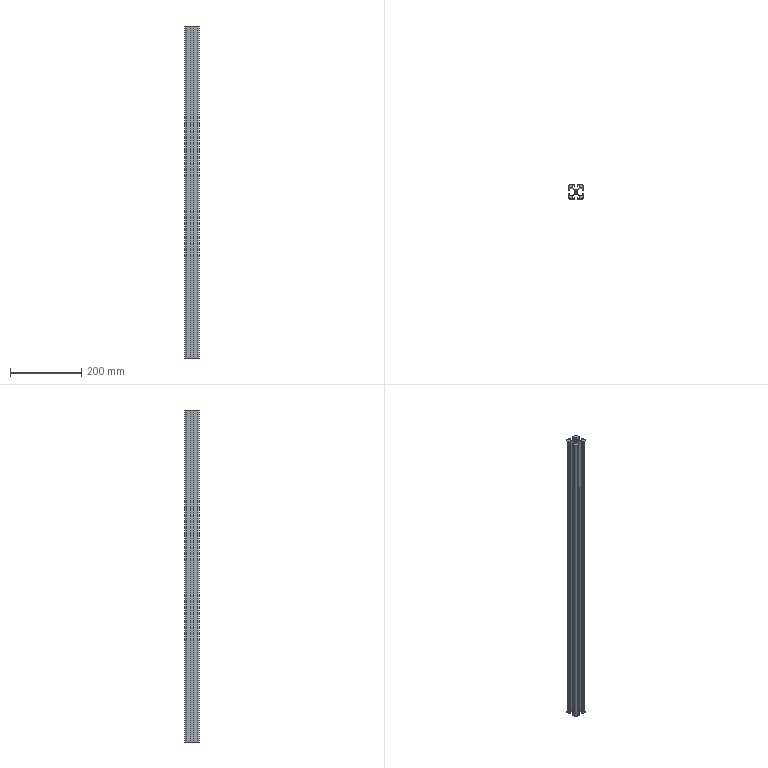Part | STEP file | 40x40-930 | 1 solid | 67 faces | box 40 x 40 x 930 mm | volume 513720 mm3 | plane 62 | cylinder 5 | commonest cylinder face diameters 9 x4 6.8 x1